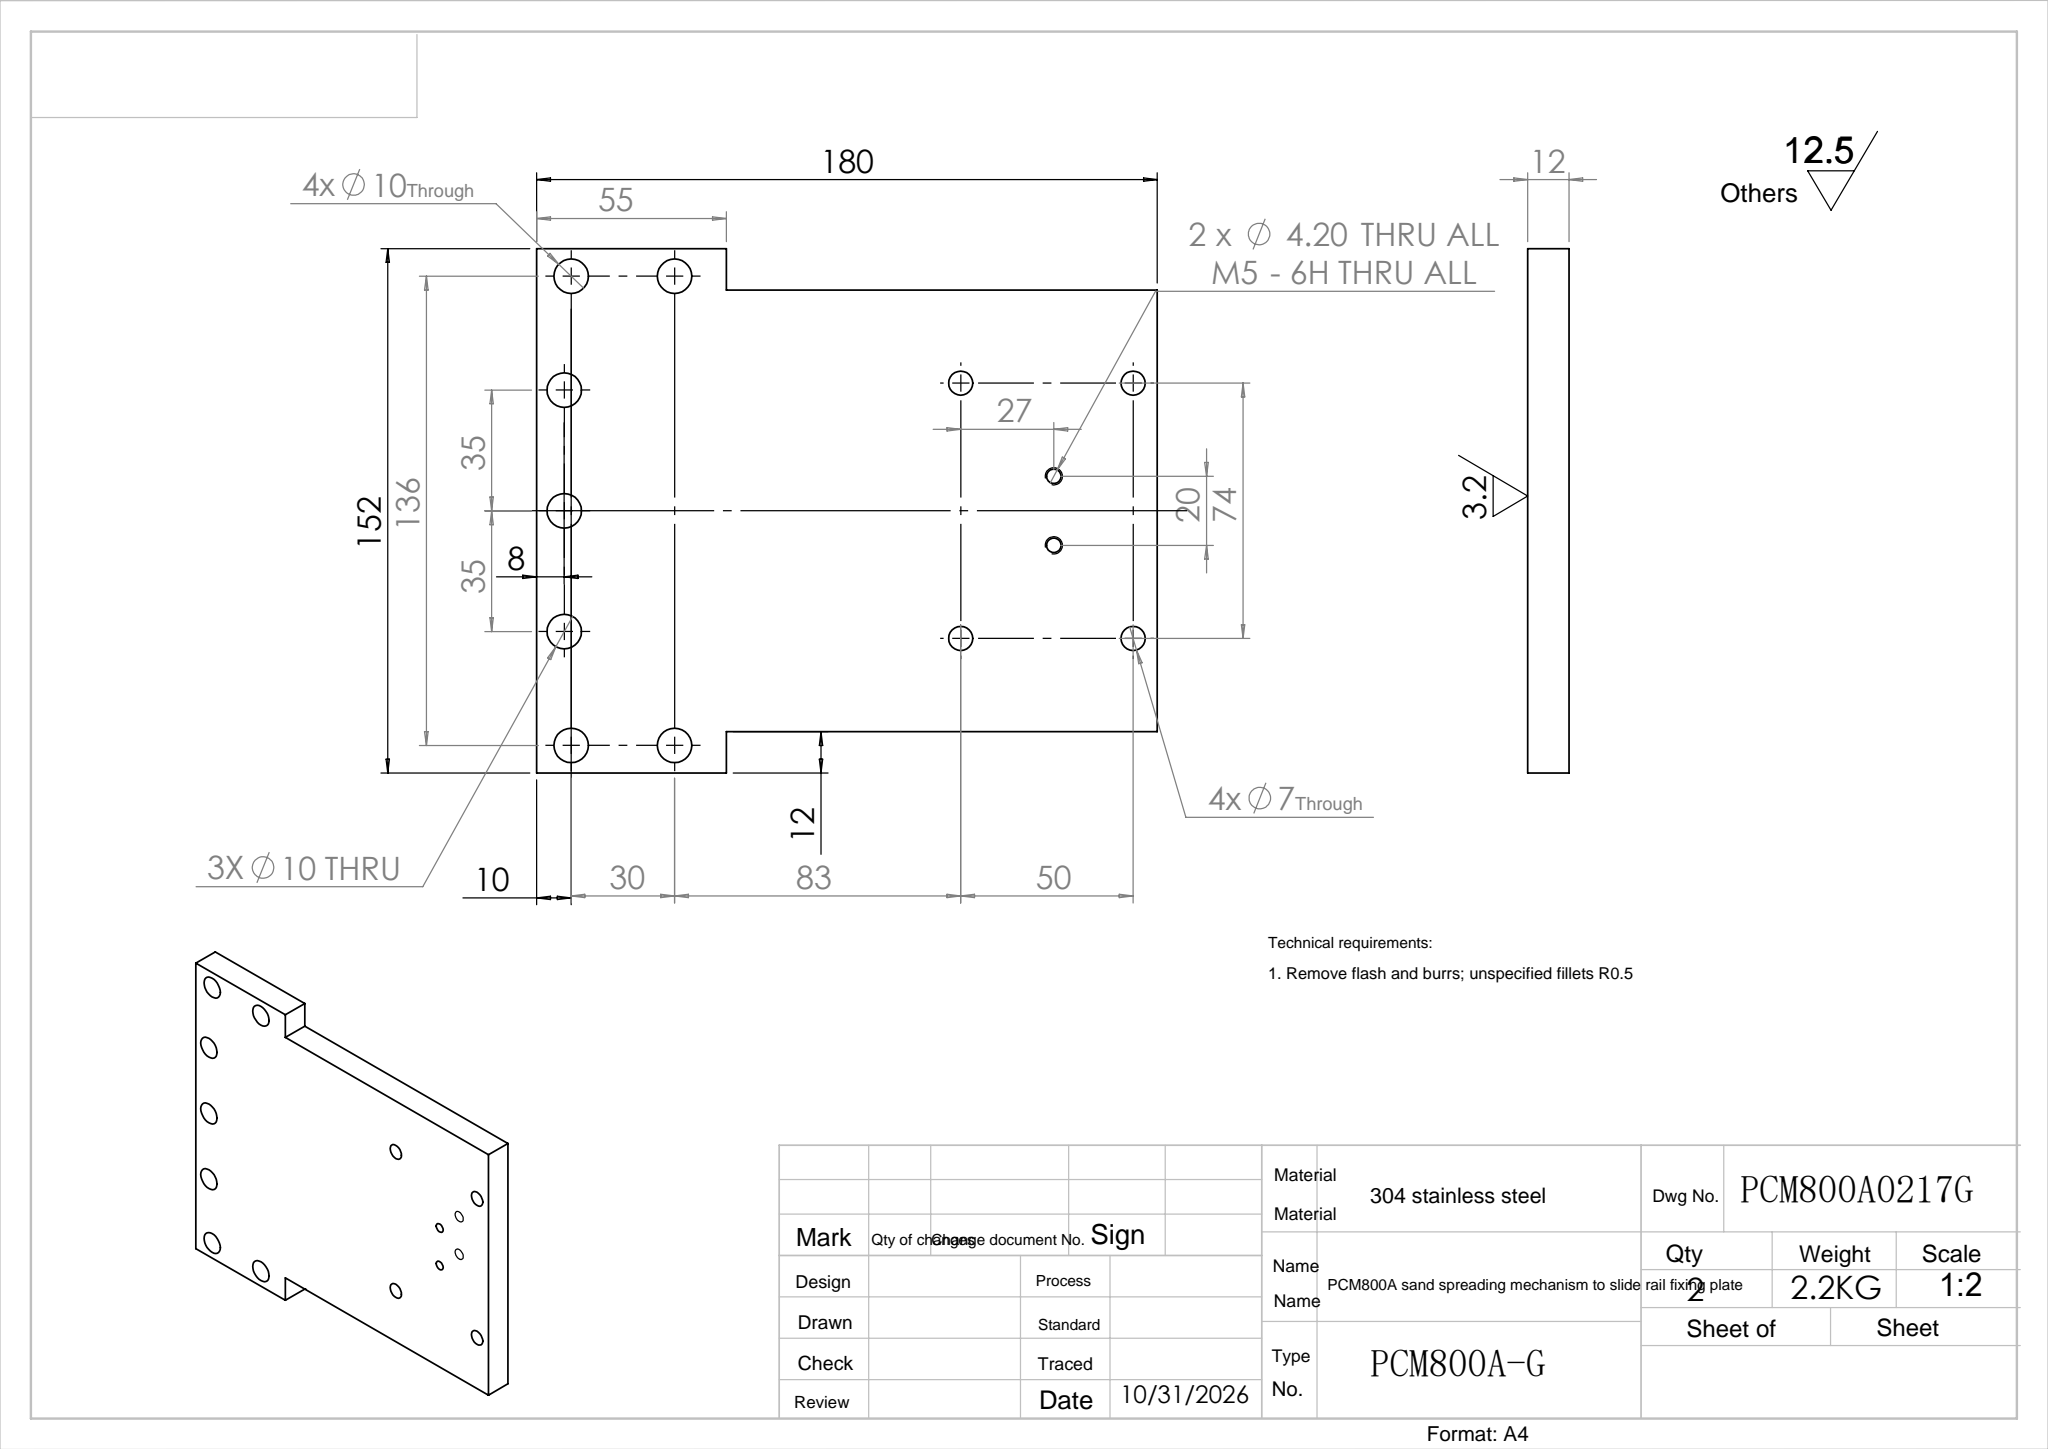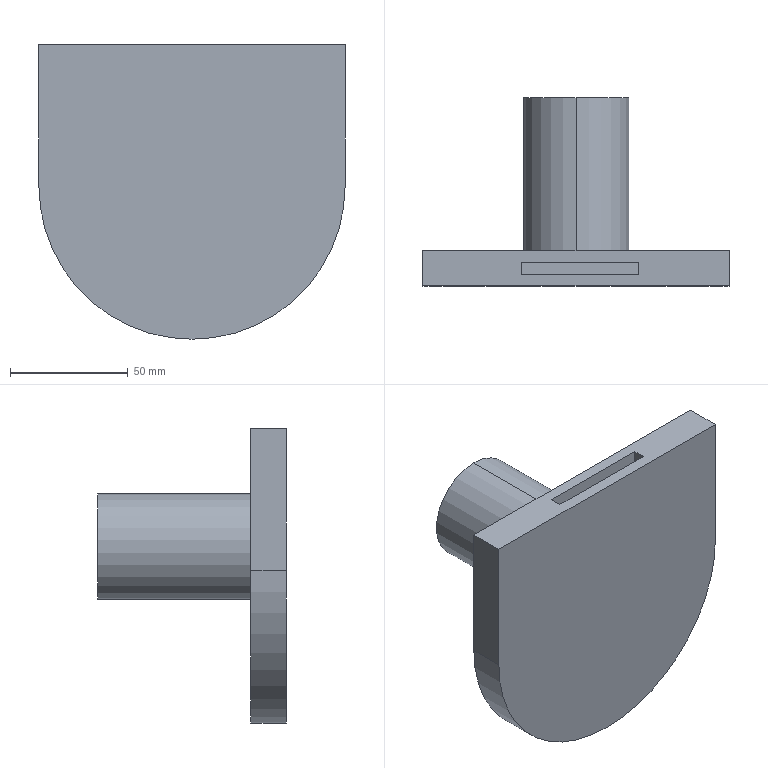Part | SolidWorks | features ICE 3, Extrusion 1 | 1 solid | 18 faces | box 130 x 80 x 125 mm | volume 284219 mm3 | plane 12 | cylinder 6 | commonest cylinder face diameters 20 x2 45 x2 130 x2
STEP:
#1=CARTESIAN_POINT('',(65.,30.,-60.));
#2=VERTEX_POINT('',#1);
#3=CARTESIAN_POINT('',(65.,30.,-40.));
#4=VERTEX_POINT('',#3);
#5=CARTESIAN_POINT('',(65.,30.,-50.));
#6=DIRECTION('',(0.,1.,0.));
#7=DIRECTION('',(0.,0.,1.));
#8=AXIS2_PLACEMENT_3D('',#5,#6,#7);
#9=CIRCLE('',#8,10.);
#10=EDGE_CURVE('',#2,#4,#9,.T.);
#11=ORIENTED_EDGE('',*,*,#10,.F.);
#12=CARTESIAN_POINT('',(65.,80.,-60.));
#13=VERTEX_POINT('',#12);
#14=CARTESIAN_POINT('',(65.,30.,-60.));
#15=DIRECTION('',(0.,1.,0.));
#16=VECTOR('',#15,1000.);
#17=LINE('',#14,#16);
#18=EDGE_CURVE('',#2,#13,#17,.T.);
#19=ORIENTED_EDGE('',*,*,#18,.T.);
#20=CARTESIAN_POINT('',(65.,80.,-40.));
#21=VERTEX_POINT('',#20);
#22=CARTESIAN_POINT('',(65.,80.,-50.));
#23=DIRECTION('',(0.,1.,0.));
#24=DIRECTION('',(0.,0.,1.));
#25=AXIS2_PLACEMENT_3D('',#22,#23,#24);
#26=CIRCLE('',#25,10.);
#27=EDGE_CURVE('',#13,#21,#26,.T.);
#28=ORIENTED_EDGE('',*,*,#27,.T.);
#29=CARTESIAN_POINT('',(65.,30.,-40.));
#30=DIRECTION('',(0.,1.,0.));
#31=VECTOR('',#30,1000.);
#32=LINE('',#29,#31);
#33=EDGE_CURVE('',#4,#21,#32,.T.);
#34=ORIENTED_EDGE('',*,*,#33,.F.);
#35=EDGE_LOOP('',(#11,#19,#28,#34));
#36=FACE_OUTER_BOUND('',#35,.T.);
#37=CARTESIAN_POINT('',(65.,30.,-50.));
#38=DIRECTION('',(0.,1.,0.));
#39=DIRECTION('',(0.,0.,1.));
#40=AXIS2_PLACEMENT_3D('',#37,#38,#39);
#41=CYLINDRICAL_SURFACE('',#40,10.);
#42=ADVANCED_FACE('',(#36),#41,.F.);
#43=CARTESIAN_POINT('',(65.,80.,-27.5));
#44=VERTEX_POINT('',#43);
#45=CARTESIAN_POINT('',(65.,80.,-72.5));
#46=VERTEX_POINT('',#45);
#47=CARTESIAN_POINT('',(65.,80.,-50.));
#48=DIRECTION('',(0.,1.,0.));
#49=DIRECTION('',(0.,0.,1.));
#50=AXIS2_PLACEMENT_3D('',#47,#48,#49);
#51=CIRCLE('',#50,22.5);
#52=EDGE_CURVE('',#44,#46,#51,.T.);
#53=ORIENTED_EDGE('',*,*,#52,.F.);
#54=CARTESIAN_POINT('',(65.,15.,-27.5));
#55=VERTEX_POINT('',#54);
#56=CARTESIAN_POINT('',(65.,80.,-27.5));
#57=DIRECTION('',(0.,-1.,0.));
#58=VECTOR('',#57,1000.);
#59=LINE('',#56,#58);
#60=EDGE_CURVE('',#44,#55,#59,.T.);
#61=ORIENTED_EDGE('',*,*,#60,.T.);
#62=CARTESIAN_POINT('',(65.,15.,-72.5));
#63=VERTEX_POINT('',#62);
#64=CARTESIAN_POINT('',(65.,15.,-50.));
#65=DIRECTION('',(0.,1.,0.));
#66=DIRECTION('',(0.,0.,1.));
#67=AXIS2_PLACEMENT_3D('',#64,#65,#66);
#68=CIRCLE('',#67,22.5);
#69=EDGE_CURVE('',#55,#63,#68,.T.);
#70=ORIENTED_EDGE('',*,*,#69,.T.);
#71=CARTESIAN_POINT('',(65.,80.,-72.5));
#72=DIRECTION('',(0.,-1.,0.));
#73=VECTOR('',#72,1000.);
#74=LINE('',#71,#73);
#75=EDGE_CURVE('',#46,#63,#74,.T.);
#76=ORIENTED_EDGE('',*,*,#75,.F.);
#77=EDGE_LOOP('',(#53,#61,#70,#76));
#78=FACE_OUTER_BOUND('',#77,.T.);
#79=CARTESIAN_POINT('',(65.,80.,-50.));
#80=DIRECTION('',(0.,-1.,0.));
#81=DIRECTION('',(0.,0.,-1.));
#82=AXIS2_PLACEMENT_3D('',#79,#80,#81);
#83=CYLINDRICAL_SURFACE('',#82,22.5);
#84=ADVANCED_FACE('',(#78),#83,.T.);
#85=CARTESIAN_POINT('',(65.,15.,-125.));
#86=VERTEX_POINT('',#85);
#87=CARTESIAN_POINT('',(0.,15.,-60.));
#88=VERTEX_POINT('',#87);
#89=CARTESIAN_POINT('',(65.,15.,-60.));
#90=DIRECTION('',(0.,1.,0.));
#91=DIRECTION('',(0.,0.,1.));
#92=AXIS2_PLACEMENT_3D('',#89,#90,#91);
#93=CIRCLE('',#92,65.);
#94=EDGE_CURVE('',#86,#88,#93,.T.);
#95=ORIENTED_EDGE('',*,*,#94,.F.);
#96=CARTESIAN_POINT('',(65.,0.,-125.));
#97=VERTEX_POINT('',#96);
#98=CARTESIAN_POINT('',(65.,15.,-125.));
#99=DIRECTION('',(0.,-1.,0.));
#100=VECTOR('',#99,1000.);
#101=LINE('',#98,#100);
#102=EDGE_CURVE('',#86,#97,#101,.T.);
#103=ORIENTED_EDGE('',*,*,#102,.T.);
#104=CARTESIAN_POINT('',(0.,0.,-60.));
#105=VERTEX_POINT('',#104);
#106=CARTESIAN_POINT('',(65.,0.,-60.));
#107=DIRECTION('',(0.,1.,0.));
#108=DIRECTION('',(0.,0.,1.));
#109=AXIS2_PLACEMENT_3D('',#106,#107,#108);
#110=CIRCLE('',#109,65.);
#111=EDGE_CURVE('',#97,#105,#110,.T.);
#112=ORIENTED_EDGE('',*,*,#111,.T.);
#113=CARTESIAN_POINT('',(0.,15.,-60.));
#114=DIRECTION('',(0.,-1.,0.));
#115=VECTOR('',#114,1000.);
#116=LINE('',#113,#115);
#117=EDGE_CURVE('',#88,#105,#116,.T.);
#118=ORIENTED_EDGE('',*,*,#117,.F.);
#119=EDGE_LOOP('',(#95,#103,#112,#118));
#120=FACE_OUTER_BOUND('',#119,.T.);
#121=CARTESIAN_POINT('',(65.,15.,-60.));
#122=DIRECTION('',(0.,-1.,0.));
#123=DIRECTION('',(0.,0.,-1.));
#124=AXIS2_PLACEMENT_3D('',#121,#122,#123);
#125=CYLINDRICAL_SURFACE('',#124,65.);
#126=ADVANCED_FACE('',(#120),#125,.T.);
#127=CARTESIAN_POINT('',(0.,15.,0.));
#128=VERTEX_POINT('',#127);
#129=CARTESIAN_POINT('',(0.,15.,0.));
#130=DIRECTION('',(0.,0.,1.));
#131=VECTOR('',#130,1000.);
#132=LINE('',#129,#131);
#133=EDGE_CURVE('',#88,#128,#132,.T.);
#134=ORIENTED_EDGE('',*,*,#133,.T.);
#135=CARTESIAN_POINT('',(130.,15.,0.));
#136=VERTEX_POINT('',#135);
#137=CARTESIAN_POINT('',(0.,15.,0.));
#138=DIRECTION('',(1.,0.,0.));
#139=VECTOR('',#138,1000.);
#140=LINE('',#137,#139);
#141=EDGE_CURVE('',#128,#136,#140,.T.);
#142=ORIENTED_EDGE('',*,*,#141,.T.);
#143=CARTESIAN_POINT('',(130.,15.,-60.));
#144=VERTEX_POINT('',#143);
#145=CARTESIAN_POINT('',(130.,15.,0.));
#146=DIRECTION('',(0.,0.,-1.));
#147=VECTOR('',#146,1000.);
#148=LINE('',#145,#147);
#149=EDGE_CURVE('',#136,#144,#148,.T.);
#150=ORIENTED_EDGE('',*,*,#149,.T.);
#151=CARTESIAN_POINT('',(65.,15.,-60.));
#152=DIRECTION('',(0.,1.,0.));
#153=DIRECTION('',(0.,0.,1.));
#154=AXIS2_PLACEMENT_3D('',#151,#152,#153);
#155=CIRCLE('',#154,65.);
#156=EDGE_CURVE('',#144,#86,#155,.T.);
#157=ORIENTED_EDGE('',*,*,#156,.T.);
#158=ORIENTED_EDGE('',*,*,#94,.T.);
#159=EDGE_LOOP('',(#134,#142,#150,#157,#158));
#160=FACE_OUTER_BOUND('',#159,.T.);
#161=CARTESIAN_POINT('',(65.,15.,-50.));
#162=DIRECTION('',(0.,1.,0.));
#163=DIRECTION('',(0.,0.,1.));
#164=AXIS2_PLACEMENT_3D('',#161,#162,#163);
#165=CIRCLE('',#164,22.5);
#166=EDGE_CURVE('',#63,#55,#165,.T.);
#167=ORIENTED_EDGE('',*,*,#166,.F.);
#168=ORIENTED_EDGE('',*,*,#69,.F.);
#169=EDGE_LOOP('',(#167,#168));
#170=FACE_BOUND('',#169,.T.);
#171=CARTESIAN_POINT('',(65.,15.,-60.));
#172=DIRECTION('',(0.,1.,0.));
#173=DIRECTION('',(0.,0.,1.));
#174=AXIS2_PLACEMENT_3D('',#171,#172,#173);
#175=PLANE('',#174);
#176=ADVANCED_FACE('',(#160,#170),#175,.T.);
#177=CARTESIAN_POINT('',(0.,0.,0.));
#178=VERTEX_POINT('',#177);
#179=CARTESIAN_POINT('',(0.,0.,0.));
#180=DIRECTION('',(0.,0.,1.));
#181=VECTOR('',#180,1000.);
#182=LINE('',#179,#181);
#183=EDGE_CURVE('',#105,#178,#182,.T.);
#184=ORIENTED_EDGE('',*,*,#183,.T.);
#185=CARTESIAN_POINT('',(0.,15.,0.));
#186=DIRECTION('',(0.,-1.,0.));
#187=VECTOR('',#186,1000.);
#188=LINE('',#185,#187);
#189=EDGE_CURVE('',#128,#178,#188,.T.);
#190=ORIENTED_EDGE('',*,*,#189,.F.);
#191=ORIENTED_EDGE('',*,*,#133,.F.);
#192=ORIENTED_EDGE('',*,*,#117,.T.);
#193=EDGE_LOOP('',(#184,#190,#191,#192));
#194=FACE_OUTER_BOUND('',#193,.T.);
#195=CARTESIAN_POINT('',(0.,15.,0.));
#196=DIRECTION('',(1.,0.,0.));
#197=DIRECTION('',(0.,0.,-1.));
#198=AXIS2_PLACEMENT_3D('',#195,#196,#197);
#199=PLANE('',#198);
#200=ADVANCED_FACE('',(#194),#199,.F.);
#201=CARTESIAN_POINT('',(41.712,5.,0.));
#202=VERTEX_POINT('',#201);
#203=CARTESIAN_POINT('',(91.712,5.,0.));
#204=VERTEX_POINT('',#203);
#205=CARTESIAN_POINT('',(41.712,5.,0.));
#206=DIRECTION('',(1.,0.,0.));
#207=VECTOR('',#206,1000.);
#208=LINE('',#205,#207);
#209=EDGE_CURVE('',#202,#204,#208,.T.);
#210=ORIENTED_EDGE('',*,*,#209,.F.);
#211=CARTESIAN_POINT('',(41.712,10.,0.));
#212=VERTEX_POINT('',#211);
#213=CARTESIAN_POINT('',(41.712,10.,0.));
#214=DIRECTION('',(0.,-1.,0.));
#215=VECTOR('',#214,1000.);
#216=LINE('',#213,#215);
#217=EDGE_CURVE('',#212,#202,#216,.T.);
#218=ORIENTED_EDGE('',*,*,#217,.F.);
#219=CARTESIAN_POINT('',(91.712,10.,0.));
#220=VERTEX_POINT('',#219);
#221=CARTESIAN_POINT('',(41.712,10.,0.));
#222=DIRECTION('',(-1.,0.,0.));
#223=VECTOR('',#222,1000.);
#224=LINE('',#221,#223);
#225=EDGE_CURVE('',#220,#212,#224,.T.);
#226=ORIENTED_EDGE('',*,*,#225,.F.);
#227=CARTESIAN_POINT('',(91.712,10.,0.));
#228=DIRECTION('',(0.,1.,0.));
#229=VECTOR('',#228,1000.);
#230=LINE('',#227,#229);
#231=EDGE_CURVE('',#204,#220,#230,.T.);
#232=ORIENTED_EDGE('',*,*,#231,.F.);
#233=EDGE_LOOP('',(#210,#218,#226,#232));
#234=FACE_BOUND('',#233,.T.);
#235=CARTESIAN_POINT('',(130.,0.,0.));
#236=VERTEX_POINT('',#235);
#237=CARTESIAN_POINT('',(0.,0.,0.));
#238=DIRECTION('',(1.,0.,0.));
#239=VECTOR('',#238,1000.);
#240=LINE('',#237,#239);
#241=EDGE_CURVE('',#178,#236,#240,.T.);
#242=ORIENTED_EDGE('',*,*,#241,.T.);
#243=CARTESIAN_POINT('',(130.,15.,0.));
#244=DIRECTION('',(0.,-1.,0.));
#245=VECTOR('',#244,1000.);
#246=LINE('',#243,#245);
#247=EDGE_CURVE('',#136,#236,#246,.T.);
#248=ORIENTED_EDGE('',*,*,#247,.F.);
#249=ORIENTED_EDGE('',*,*,#141,.F.);
#250=ORIENTED_EDGE('',*,*,#189,.T.);
#251=EDGE_LOOP('',(#242,#248,#249,#250));
#252=FACE_OUTER_BOUND('',#251,.T.);
#253=CARTESIAN_POINT('',(0.,15.,0.));
#254=DIRECTION('',(0.,0.,-1.));
#255=DIRECTION('',(-1.,0.,0.));
#256=AXIS2_PLACEMENT_3D('',#253,#254,#255);
#257=PLANE('',#256);
#258=ADVANCED_FACE('',(#234,#252),#257,.F.);
#259=CARTESIAN_POINT('',(130.,0.,-60.));
#260=VERTEX_POINT('',#259);
#261=CARTESIAN_POINT('',(130.,0.,0.));
#262=DIRECTION('',(0.,0.,-1.));
#263=VECTOR('',#262,1000.);
#264=LINE('',#261,#263);
#265=EDGE_CURVE('',#236,#260,#264,.T.);
#266=ORIENTED_EDGE('',*,*,#265,.T.);
#267=CARTESIAN_POINT('',(130.,15.,-60.));
#268=DIRECTION('',(0.,-1.,0.));
#269=VECTOR('',#268,1000.);
#270=LINE('',#267,#269);
#271=EDGE_CURVE('',#144,#260,#270,.T.);
#272=ORIENTED_EDGE('',*,*,#271,.F.);
#273=ORIENTED_EDGE('',*,*,#149,.F.);
#274=ORIENTED_EDGE('',*,*,#247,.T.);
#275=EDGE_LOOP('',(#266,#272,#273,#274));
#276=FACE_OUTER_BOUND('',#275,.T.);
#277=CARTESIAN_POINT('',(130.,15.,0.));
#278=DIRECTION('',(-1.,0.,0.));
#279=DIRECTION('',(0.,0.,1.));
#280=AXIS2_PLACEMENT_3D('',#277,#278,#279);
#281=PLANE('',#280);
#282=ADVANCED_FACE('',(#276),#281,.F.);
#283=ORIENTED_EDGE('',*,*,#102,.F.);
#284=ORIENTED_EDGE('',*,*,#156,.F.);
#285=ORIENTED_EDGE('',*,*,#271,.T.);
#286=CARTESIAN_POINT('',(65.,0.,-60.));
#287=DIRECTION('',(0.,1.,0.));
#288=DIRECTION('',(0.,0.,1.));
#289=AXIS2_PLACEMENT_3D('',#286,#287,#288);
#290=CIRCLE('',#289,65.);
#291=EDGE_CURVE('',#260,#97,#290,.T.);
#292=ORIENTED_EDGE('',*,*,#291,.T.);
#293=EDGE_LOOP('',(#283,#284,#285,#292));
#294=FACE_OUTER_BOUND('',#293,.T.);
#295=CARTESIAN_POINT('',(65.,15.,-60.));
#296=DIRECTION('',(0.,-1.,0.));
#297=DIRECTION('',(0.,0.,-1.));
#298=AXIS2_PLACEMENT_3D('',#295,#296,#297);
#299=CYLINDRICAL_SURFACE('',#298,65.);
#300=ADVANCED_FACE('',(#294),#299,.T.);
#301=ORIENTED_EDGE('',*,*,#183,.F.);
#302=ORIENTED_EDGE('',*,*,#111,.F.);
#303=ORIENTED_EDGE('',*,*,#291,.F.);
#304=ORIENTED_EDGE('',*,*,#265,.F.);
#305=ORIENTED_EDGE('',*,*,#241,.F.);
#306=EDGE_LOOP('',(#301,#302,#303,#304,#305));
#307=FACE_OUTER_BOUND('',#306,.T.);
#308=CARTESIAN_POINT('',(65.,0.,-60.));
#309=DIRECTION('',(0.,1.,0.));
#310=DIRECTION('',(0.,0.,1.));
#311=AXIS2_PLACEMENT_3D('',#308,#309,#310);
#312=PLANE('',#311);
#313=ADVANCED_FACE('',(#307),#312,.F.);
#314=ORIENTED_EDGE('',*,*,#60,.F.);
#315=CARTESIAN_POINT('',(65.,80.,-50.));
#316=DIRECTION('',(0.,1.,0.));
#317=DIRECTION('',(0.,0.,1.));
#318=AXIS2_PLACEMENT_3D('',#315,#316,#317);
#319=CIRCLE('',#318,22.5);
#320=EDGE_CURVE('',#46,#44,#319,.T.);
#321=ORIENTED_EDGE('',*,*,#320,.F.);
#322=ORIENTED_EDGE('',*,*,#75,.T.);
#323=ORIENTED_EDGE('',*,*,#166,.T.);
#324=EDGE_LOOP('',(#314,#321,#322,#323));
#325=FACE_OUTER_BOUND('',#324,.T.);
#326=CARTESIAN_POINT('',(65.,80.,-50.));
#327=DIRECTION('',(0.,-1.,0.));
#328=DIRECTION('',(0.,0.,-1.));
#329=AXIS2_PLACEMENT_3D('',#326,#327,#328);
#330=CYLINDRICAL_SURFACE('',#329,22.5);
#331=ADVANCED_FACE('',(#325),#330,.T.);
#332=CARTESIAN_POINT('',(65.,80.,-50.));
#333=DIRECTION('',(0.,1.,0.));
#334=DIRECTION('',(0.,0.,1.));
#335=AXIS2_PLACEMENT_3D('',#332,#333,#334);
#336=CIRCLE('',#335,10.);
#337=EDGE_CURVE('',#21,#13,#336,.T.);
#338=ORIENTED_EDGE('',*,*,#337,.F.);
#339=ORIENTED_EDGE('',*,*,#27,.F.);
#340=EDGE_LOOP('',(#338,#339));
#341=FACE_BOUND('',#340,.T.);
#342=ORIENTED_EDGE('',*,*,#320,.T.);
#343=ORIENTED_EDGE('',*,*,#52,.T.);
#344=EDGE_LOOP('',(#342,#343));
#345=FACE_OUTER_BOUND('',#344,.T.);
#346=CARTESIAN_POINT('',(65.,80.,-50.));
#347=DIRECTION('',(0.,1.,0.));
#348=DIRECTION('',(0.,0.,1.));
#349=AXIS2_PLACEMENT_3D('',#346,#347,#348);
#350=PLANE('',#349);
#351=ADVANCED_FACE('',(#341,#345),#350,.T.);
#352=ORIENTED_EDGE('',*,*,#217,.T.);
#353=CARTESIAN_POINT('',(41.712,5.,-80.));
#354=VERTEX_POINT('',#353);
#355=CARTESIAN_POINT('',(41.712,5.,-80.));
#356=DIRECTION('',(0.,0.,1.));
#357=VECTOR('',#356,1000.);
#358=LINE('',#355,#357);
#359=EDGE_CURVE('',#354,#202,#358,.T.);
#360=ORIENTED_EDGE('',*,*,#359,.F.);
#361=CARTESIAN_POINT('',(41.712,10.,-80.));
#362=VERTEX_POINT('',#361);
#363=CARTESIAN_POINT('',(41.712,10.,-80.));
#364=DIRECTION('',(0.,-1.,0.));
#365=VECTOR('',#364,1000.);
#366=LINE('',#363,#365);
#367=EDGE_CURVE('',#362,#354,#366,.T.);
#368=ORIENTED_EDGE('',*,*,#367,.F.);
#369=CARTESIAN_POINT('',(41.712,10.,-80.));
#370=DIRECTION('',(0.,0.,1.));
#371=VECTOR('',#370,1000.);
#372=LINE('',#369,#371);
#373=EDGE_CURVE('',#362,#212,#372,.T.);
#374=ORIENTED_EDGE('',*,*,#373,.T.);
#375=EDGE_LOOP('',(#352,#360,#368,#374));
#376=FACE_OUTER_BOUND('',#375,.T.);
#377=CARTESIAN_POINT('',(41.712,10.,-80.));
#378=DIRECTION('',(-1.,0.,0.));
#379=DIRECTION('',(0.,0.,1.));
#380=AXIS2_PLACEMENT_3D('',#377,#378,#379);
#381=PLANE('',#380);
#382=ADVANCED_FACE('',(#376),#381,.F.);
#383=ORIENTED_EDGE('',*,*,#225,.T.);
#384=ORIENTED_EDGE('',*,*,#373,.F.);
#385=CARTESIAN_POINT('',(91.712,10.,-80.));
#386=VERTEX_POINT('',#385);
#387=CARTESIAN_POINT('',(41.712,10.,-80.));
#388=DIRECTION('',(-1.,0.,0.));
#389=VECTOR('',#388,1000.);
#390=LINE('',#387,#389);
#391=EDGE_CURVE('',#386,#362,#390,.T.);
#392=ORIENTED_EDGE('',*,*,#391,.F.);
#393=CARTESIAN_POINT('',(91.712,10.,-80.));
#394=DIRECTION('',(0.,0.,1.));
#395=VECTOR('',#394,1000.);
#396=LINE('',#393,#395);
#397=EDGE_CURVE('',#386,#220,#396,.T.);
#398=ORIENTED_EDGE('',*,*,#397,.T.);
#399=EDGE_LOOP('',(#383,#384,#392,#398));
#400=FACE_OUTER_BOUND('',#399,.T.);
#401=CARTESIAN_POINT('',(41.712,10.,-80.));
#402=DIRECTION('',(0.,1.,0.));
#403=DIRECTION('',(-1.,0.,0.));
#404=AXIS2_PLACEMENT_3D('',#401,#402,#403);
#405=PLANE('',#404);
#406=ADVANCED_FACE('',(#400),#405,.F.);
#407=ORIENTED_EDGE('',*,*,#231,.T.);
#408=ORIENTED_EDGE('',*,*,#397,.F.);
#409=CARTESIAN_POINT('',(91.712,5.,-80.));
#410=VERTEX_POINT('',#409);
#411=CARTESIAN_POINT('',(91.712,10.,-80.));
#412=DIRECTION('',(0.,1.,0.));
#413=VECTOR('',#412,1000.);
#414=LINE('',#411,#413);
#415=EDGE_CURVE('',#410,#386,#414,.T.);
#416=ORIENTED_EDGE('',*,*,#415,.F.);
#417=CARTESIAN_POINT('',(91.712,5.,-80.));
#418=DIRECTION('',(0.,0.,1.));
#419=VECTOR('',#418,1000.);
#420=LINE('',#417,#419);
#421=EDGE_CURVE('',#410,#204,#420,.T.);
#422=ORIENTED_EDGE('',*,*,#421,.T.);
#423=EDGE_LOOP('',(#407,#408,#416,#422));
#424=FACE_OUTER_BOUND('',#423,.T.);
#425=CARTESIAN_POINT('',(91.712,10.,-80.));
#426=DIRECTION('',(1.,0.,0.));
#427=DIRECTION('',(0.,0.,-1.));
#428=AXIS2_PLACEMENT_3D('',#425,#426,#427);
#429=PLANE('',#428);
#430=ADVANCED_FACE('',(#424),#429,.F.);
#431=ORIENTED_EDGE('',*,*,#209,.T.);
#432=ORIENTED_EDGE('',*,*,#421,.F.);
#433=CARTESIAN_POINT('',(41.712,5.,-80.));
#434=DIRECTION('',(1.,0.,0.));
#435=VECTOR('',#434,1000.);
#436=LINE('',#433,#435);
#437=EDGE_CURVE('',#354,#410,#436,.T.);
#438=ORIENTED_EDGE('',*,*,#437,.F.);
#439=ORIENTED_EDGE('',*,*,#359,.T.);
#440=EDGE_LOOP('',(#431,#432,#438,#439));
#441=FACE_OUTER_BOUND('',#440,.T.);
#442=CARTESIAN_POINT('',(41.712,5.,-80.));
#443=DIRECTION('',(0.,-1.,0.));
#444=DIRECTION('',(0.,0.,-1.));
#445=AXIS2_PLACEMENT_3D('',#442,#443,#444);
#446=PLANE('',#445);
#447=ADVANCED_FACE('',(#441),#446,.F.);
#448=ORIENTED_EDGE('',*,*,#367,.T.);
#449=ORIENTED_EDGE('',*,*,#437,.T.);
#450=ORIENTED_EDGE('',*,*,#415,.T.);
#451=ORIENTED_EDGE('',*,*,#391,.T.);
#452=EDGE_LOOP('',(#448,#449,#450,#451));
#453=FACE_OUTER_BOUND('',#452,.T.);
#454=CARTESIAN_POINT('',(41.712,5.,-80.));
#455=DIRECTION('',(0.,0.,1.));
#456=DIRECTION('',(1.,0.,0.));
#457=AXIS2_PLACEMENT_3D('',#454,#455,#456);
#458=PLANE('',#457);
#459=ADVANCED_FACE('',(#453),#458,.T.);
#460=ORIENTED_EDGE('',*,*,#18,.F.);
#461=CARTESIAN_POINT('',(65.,30.,-50.));
#462=DIRECTION('',(0.,1.,0.));
#463=DIRECTION('',(0.,0.,1.));
#464=AXIS2_PLACEMENT_3D('',#461,#462,#463);
#465=CIRCLE('',#464,10.);
#466=EDGE_CURVE('',#4,#2,#465,.T.);
#467=ORIENTED_EDGE('',*,*,#466,.F.);
#468=ORIENTED_EDGE('',*,*,#33,.T.);
#469=ORIENTED_EDGE('',*,*,#337,.T.);
#470=EDGE_LOOP('',(#460,#467,#468,#469));
#471=FACE_OUTER_BOUND('',#470,.T.);
#472=CARTESIAN_POINT('',(65.,30.,-50.));
#473=DIRECTION('',(0.,1.,0.));
#474=DIRECTION('',(0.,0.,1.));
#475=AXIS2_PLACEMENT_3D('',#472,#473,#474);
#476=CYLINDRICAL_SURFACE('',#475,10.);
#477=ADVANCED_FACE('',(#471),#476,.F.);
#478=ORIENTED_EDGE('',*,*,#466,.T.);
#479=ORIENTED_EDGE('',*,*,#10,.T.);
#480=EDGE_LOOP('',(#478,#479));
#481=FACE_OUTER_BOUND('',#480,.T.);
#482=CARTESIAN_POINT('',(65.,30.,-50.));
#483=DIRECTION('',(0.,1.,0.));
#484=DIRECTION('',(0.,0.,1.));
#485=AXIS2_PLACEMENT_3D('',#482,#483,#484);
#486=PLANE('',#485);
#487=ADVANCED_FACE('',(#481),#486,.T.);
#488=CLOSED_SHELL('',(#42,#84,#126,#176,#200,#258,#282,#300,#313,#331,#351,#382,#406,#430,#447,#459,#477,#487));
#489=MANIFOLD_SOLID_BREP('',#488);
#490=CARTESIAN_POINT('',(0.,0.,0.));
#491=DIRECTION('',(0.,0.,1.));
#492=DIRECTION('',(1.,0.,0.));
#493=AXIS2_PLACEMENT_3D('',#490,#491,#492);
#494=(LENGTH_UNIT()NAMED_UNIT(*)SI_UNIT(.MILLI.,.METRE.));
#495=UNCERTAINTY_MEASURE_WITH_UNIT(LENGTH_MEASURE(0.00001),#494,'','');
#496=(NAMED_UNIT(*)PLANE_ANGLE_UNIT()SI_UNIT($,.RADIAN.));
#497=(NAMED_UNIT(*)SI_UNIT($,.STERADIAN.)SOLID_ANGLE_UNIT());
#498=(GEOMETRIC_REPRESENTATION_CONTEXT(3)GLOBAL_UNCERTAINTY_ASSIGNED_CONTEXT((#495))GLOBAL_UNIT_ASSIGNED_CONTEXT((#494,#496,#497))REPRESENTATION_CONTEXT('',''));
#499=ADVANCED_BREP_SHAPE_REPRESENTATION('',(#489,#493),#498);